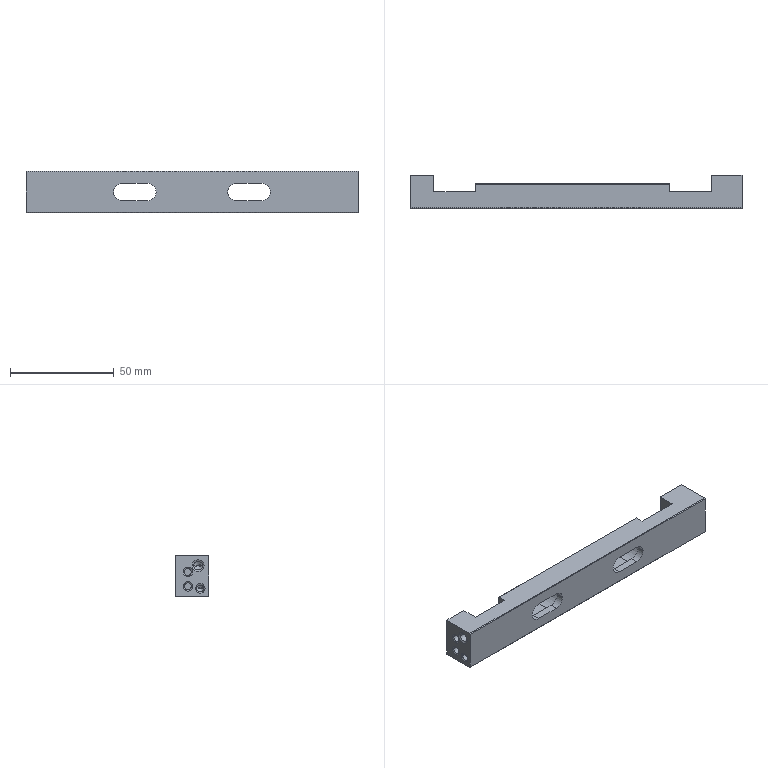Part | NX | 1 solid | 60 faces | box 160 x 16 x 20 mm | volume 29819 mm3 | plane 28 | cylinder 20 | cone 12 | commonest cylinder face diameters 3.3 x6 8.5 x6 14.5 x6 4.2 x2